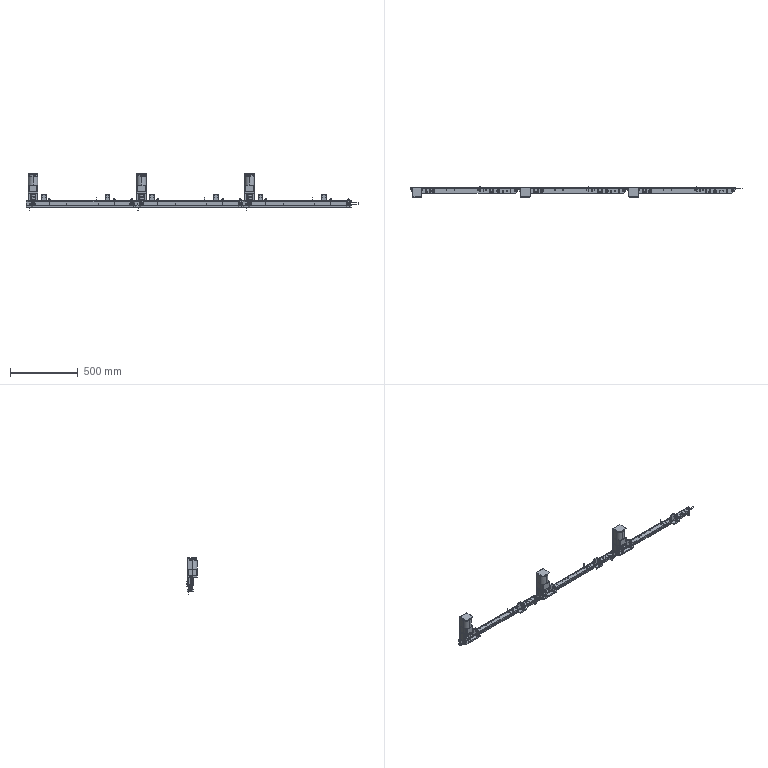Part | NX | 177 solids | 6015 faces | volume 4125877 mm3 | cylinder 2706 | cone 1560 | plane 1521 | torus 186 | spline 42 | commonest cylinder face diameters 2.5 x402 3.3 x390 4.2 x210 3.5 x180 6 x174 5.5 x168